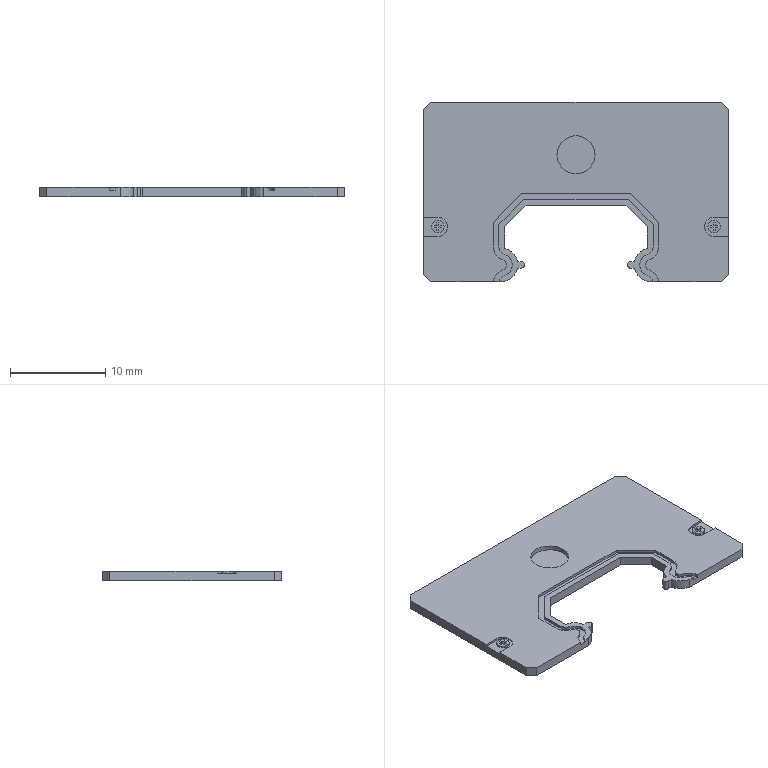Part | STEP file | 12 | 1 solid | 99 faces | box 32 x 18.8 x 1 mm | volume 479.678 mm3 | plane 69 | cylinder 30 | commonest cylinder face diameters 1.3 x4 1.9 x4 3.1 x4 3.5 x4 0.7 x3 1.1 x3